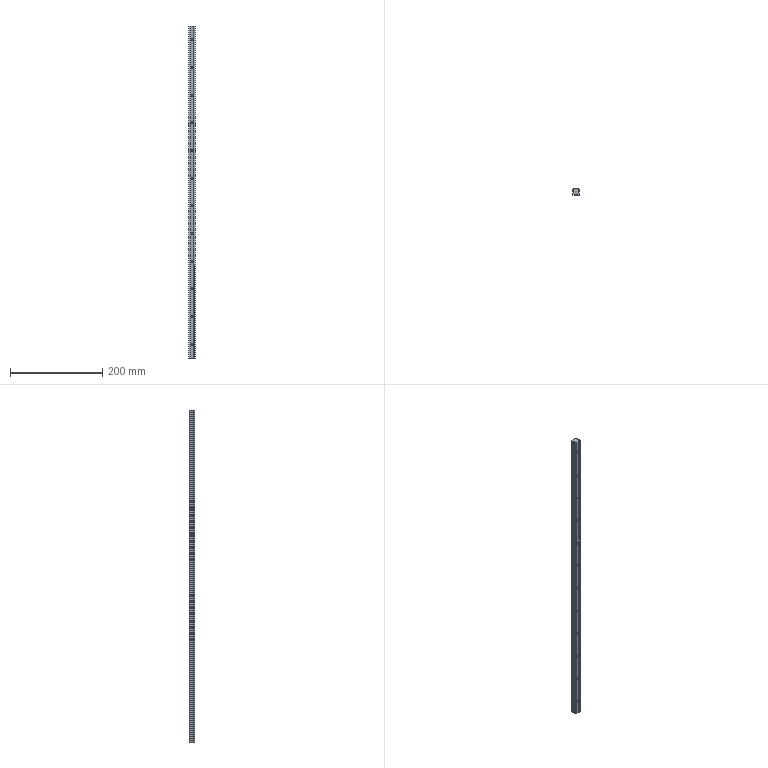Part | SolidWorks | features Fillet 8, ICE 4, Chamfer 2, Extrusion 1, HoleWzd 1, LPattern 1 | 1 solid | 96 faces | box 15 x 13 x 720 mm | volume 116945 mm3 | cylinder 61 | plane 35 | commonest cylinder face diameters 4.5 x24 7.5 x24 0.6 x8 2.6 x4 1 x1